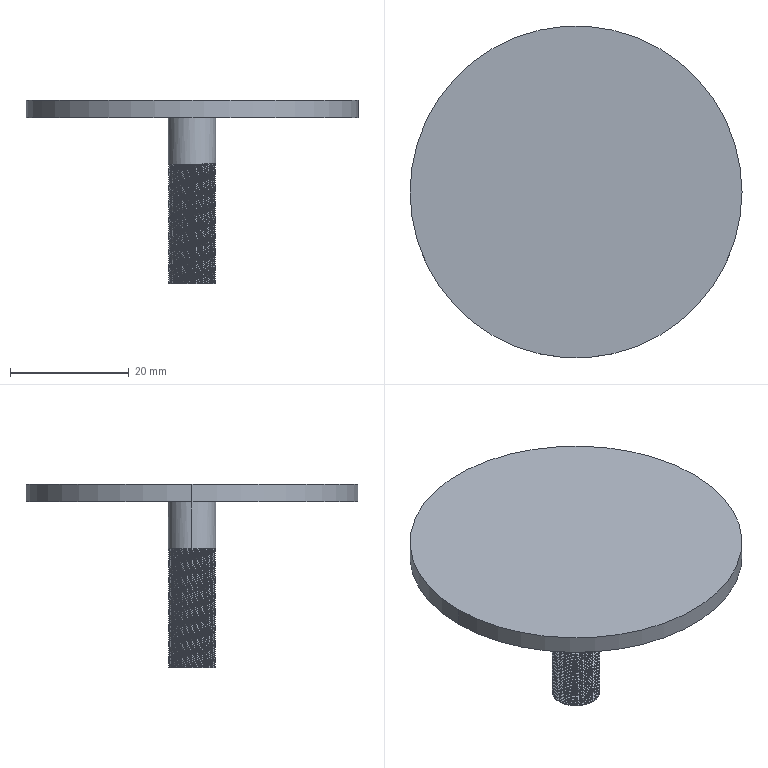Part | SolidWorks | features Extrusion 1, ICE 1, SweepThread 1 | 1 solid | 137 faces | box 56 x 56 x 31 mm | volume 8748 mm3 | cylinder 129 | plane 5 | spline 3 | commonest cylinder face diameters 8 x127 56 x2